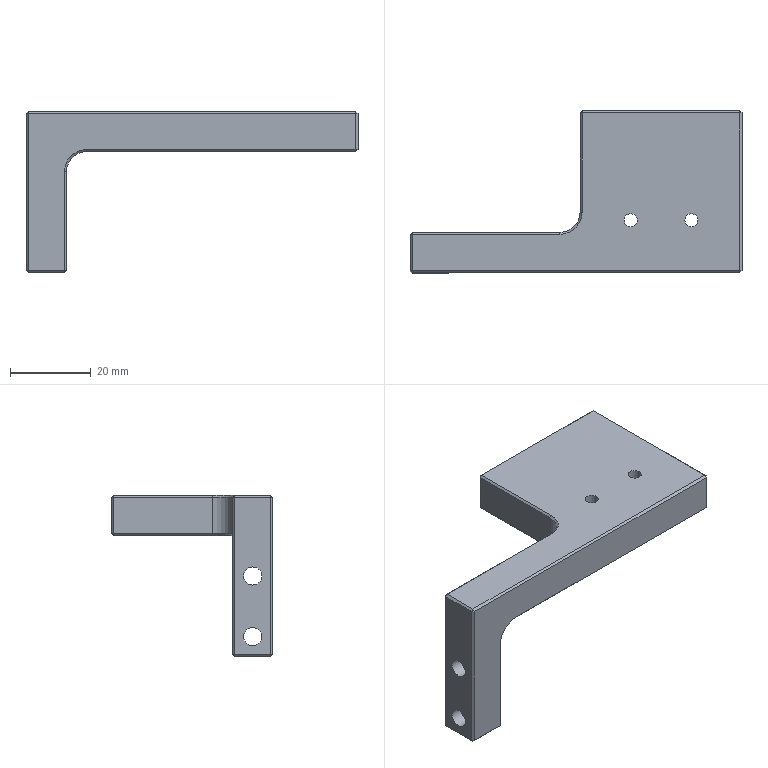Part | 1 solid | 54 faces | box 82 x 40 x 40 mm | volume 22743 mm3 | plane 44 | cylinder 6 | cone 4 | commonest cylinder face diameters 3.242 x2 4.5 x2 10 x2
STEP:
#1=CARTESIAN_POINT('',(11.879,-7.,-10.));
#2=VERTEX_POINT('',#1);
#3=CARTESIAN_POINT('',(13.5,-7.,-10.));
#4=DIRECTION('',(0.,0.,-1.));
#5=DIRECTION('',(-1.,0.,0.));
#6=AXIS2_PLACEMENT_3D('',#3,#4,#5);
#7=CIRCLE('',#6,1.621);
#8=EDGE_CURVE('',#2,#2,#7,.T.);
#9=ORIENTED_EDGE('',*,*,#8,.T.);
#10=EDGE_LOOP('',(#9));
#11=FACE_BOUND('',#10,.T.);
#12=CARTESIAN_POINT('',(15.121,-7.,0.));
#13=VERTEX_POINT('',#12);
#14=CARTESIAN_POINT('',(13.5,-7.,0.));
#15=DIRECTION('',(0.,0.,1.));
#16=DIRECTION('',(1.,0.,0.));
#17=AXIS2_PLACEMENT_3D('',#14,#15,#16);
#18=CIRCLE('',#17,1.621);
#19=EDGE_CURVE('',#13,#13,#18,.T.);
#20=ORIENTED_EDGE('',*,*,#19,.T.);
#21=EDGE_LOOP('',(#20));
#22=FACE_BOUND('',#21,.T.);
#23=CARTESIAN_POINT('',(13.5,-7.,0.));
#24=DIRECTION('',(0.,0.,-1.));
#25=DIRECTION('',(1.,0.,0.));
#26=AXIS2_PLACEMENT_3D('',#23,#24,#25);
#27=CYLINDRICAL_SURFACE('',#26,1.621);
#28=ADVANCED_FACE('',(#11,#22),#27,.F.);
#29=CARTESIAN_POINT('',(1.5,19.5,-10.));
#30=VERTEX_POINT('',#29);
#31=CARTESIAN_POINT('',(1.5,20.,-9.5));
#32=VERTEX_POINT('',#31);
#33=CARTESIAN_POINT('',(1.5,19.75,-9.75));
#34=DIRECTION('',(0.,0.7071,0.7071));
#35=VECTOR('',#34,1000.);
#36=LINE('',#33,#35);
#37=EDGE_CURVE('',#30,#32,#36,.T.);
#38=ORIENTED_EDGE('',*,*,#37,.T.);
#39=CARTESIAN_POINT('',(40.5,20.,-9.5));
#40=VERTEX_POINT('',#39);
#41=CARTESIAN_POINT('',(21.,20.,-9.5));
#42=DIRECTION('',(-1.,0.,0.));
#43=VECTOR('',#42,1000.);
#44=LINE('',#41,#43);
#45=EDGE_CURVE('',#40,#32,#44,.T.);
#46=ORIENTED_EDGE('',*,*,#45,.F.);
#47=CARTESIAN_POINT('',(40.5,19.5,-10.));
#48=VERTEX_POINT('',#47);
#49=CARTESIAN_POINT('',(40.5,19.75,-9.75));
#50=DIRECTION('',(0.,-0.7071,-0.7071));
#51=VECTOR('',#50,1000.);
#52=LINE('',#49,#51);
#53=EDGE_CURVE('',#40,#48,#52,.T.);
#54=ORIENTED_EDGE('',*,*,#53,.T.);
#55=CARTESIAN_POINT('',(21.,19.5,-10.));
#56=DIRECTION('',(-1.,0.,0.));
#57=VECTOR('',#56,1000.);
#58=LINE('',#55,#57);
#59=EDGE_CURVE('',#48,#30,#58,.T.);
#60=ORIENTED_EDGE('',*,*,#59,.T.);
#61=EDGE_LOOP('',(#38,#46,#54,#60));
#62=FACE_BOUND('',#61,.T.);
#63=CARTESIAN_POINT('',(7.25,20.,-9.5));
#64=DIRECTION('',(0.,-0.7071,0.7071));
#65=DIRECTION('',(-1.,0.,0.));
#66=AXIS2_PLACEMENT_3D('',#63,#64,#65);
#67=PLANE('',#66);
#68=ADVANCED_FACE('',(#62),#67,.F.);
#69=CARTESIAN_POINT('',(41.,19.5,-9.5));
#70=VERTEX_POINT('',#69);
#71=CARTESIAN_POINT('',(40.75,19.5,-9.75));
#72=DIRECTION('',(0.7071,0.,0.7071));
#73=VECTOR('',#72,1000.);
#74=LINE('',#71,#73);
#75=EDGE_CURVE('',#48,#70,#74,.T.);
#76=ORIENTED_EDGE('',*,*,#75,.T.);
#77=CARTESIAN_POINT('',(41.,-19.5,-9.5));
#78=VERTEX_POINT('',#77);
#79=CARTESIAN_POINT('',(41.,0.,-9.5));
#80=DIRECTION('',(0.,1.,0.));
#81=VECTOR('',#80,1000.);
#82=LINE('',#79,#81);
#83=EDGE_CURVE('',#78,#70,#82,.T.);
#84=ORIENTED_EDGE('',*,*,#83,.F.);
#85=CARTESIAN_POINT('',(40.5,-19.5,-10.));
#86=VERTEX_POINT('',#85);
#87=CARTESIAN_POINT('',(40.75,-19.5,-9.75));
#88=DIRECTION('',(-0.7071,0.,-0.7071));
#89=VECTOR('',#88,1000.);
#90=LINE('',#87,#89);
#91=EDGE_CURVE('',#78,#86,#90,.T.);
#92=ORIENTED_EDGE('',*,*,#91,.T.);
#93=CARTESIAN_POINT('',(40.5,0.,-10.));
#94=DIRECTION('',(0.,1.,0.));
#95=VECTOR('',#94,1000.);
#96=LINE('',#93,#95);
#97=EDGE_CURVE('',#86,#48,#96,.T.);
#98=ORIENTED_EDGE('',*,*,#97,.T.);
#99=EDGE_LOOP('',(#76,#84,#92,#98));
#100=FACE_BOUND('',#99,.T.);
#101=CARTESIAN_POINT('',(41.,0.25,-9.5));
#102=DIRECTION('',(-0.7071,0.,0.7071));
#103=DIRECTION('',(0.,1.,0.));
#104=AXIS2_PLACEMENT_3D('',#101,#102,#103);
#105=PLANE('',#104);
#106=ADVANCED_FACE('',(#100),#105,.F.);
#107=CARTESIAN_POINT('',(40.5,-20.,-9.5));
#108=VERTEX_POINT('',#107);
#109=CARTESIAN_POINT('',(-26.,-20.,-9.5));
#110=VERTEX_POINT('',#109);
#111=CARTESIAN_POINT('',(7.25,-20.,-9.5));
#112=DIRECTION('',(-1.,0.,0.));
#113=VECTOR('',#112,1000.);
#114=LINE('',#111,#113);
#115=EDGE_CURVE('',#108,#110,#114,.T.);
#116=ORIENTED_EDGE('',*,*,#115,.T.);
#117=CARTESIAN_POINT('',(-26.,-19.5,-10.));
#118=VERTEX_POINT('',#117);
#119=CARTESIAN_POINT('',(-26.,-19.75,-9.75));
#120=DIRECTION('',(0.,-0.7071,0.7071));
#121=VECTOR('',#120,1000.);
#122=LINE('',#119,#121);
#123=EDGE_CURVE('',#118,#110,#122,.T.);
#124=ORIENTED_EDGE('',*,*,#123,.F.);
#125=CARTESIAN_POINT('',(7.25,-19.5,-10.));
#126=DIRECTION('',(-1.,0.,0.));
#127=VECTOR('',#126,1000.);
#128=LINE('',#125,#127);
#129=EDGE_CURVE('',#86,#118,#128,.T.);
#130=ORIENTED_EDGE('',*,*,#129,.F.);
#131=CARTESIAN_POINT('',(40.5,-19.75,-9.75));
#132=DIRECTION('',(0.,-0.7071,0.7071));
#133=VECTOR('',#132,1000.);
#134=LINE('',#131,#133);
#135=EDGE_CURVE('',#86,#108,#134,.T.);
#136=ORIENTED_EDGE('',*,*,#135,.T.);
#137=EDGE_LOOP('',(#116,#124,#130,#136));
#138=FACE_BOUND('',#137,.T.);
#139=CARTESIAN_POINT('',(0.,-20.,-9.5));
#140=DIRECTION('',(0.,-0.7071,-0.7071));
#141=DIRECTION('',(-1.,0.,0.));
#142=AXIS2_PLACEMENT_3D('',#139,#140,#141);
#143=PLANE('',#142);
#144=ADVANCED_FACE('',(#138),#143,.T.);
#145=CARTESIAN_POINT('',(-31.,-10.5,-15.));
#146=VERTEX_POINT('',#145);
#147=CARTESIAN_POINT('',(-26.,-10.5,-10.));
#148=VERTEX_POINT('',#147);
#149=CARTESIAN_POINT('',(-26.,-10.5,-15.));
#150=DIRECTION('',(0.,1.,0.));
#151=DIRECTION('',(1.,0.,0.));
#152=AXIS2_PLACEMENT_3D('',#149,#150,#151);
#153=CIRCLE('',#152,5.);
#154=EDGE_CURVE('',#146,#148,#153,.T.);
#155=ORIENTED_EDGE('',*,*,#154,.T.);
#156=CARTESIAN_POINT('',(-26.,-15.,-10.));
#157=DIRECTION('',(0.,1.,0.));
#158=VECTOR('',#157,1000.);
#159=LINE('',#156,#158);
#160=EDGE_CURVE('',#118,#148,#159,.T.);
#161=ORIENTED_EDGE('',*,*,#160,.F.);
#162=CARTESIAN_POINT('',(-31.,-19.5,-15.));
#163=VERTEX_POINT('',#162);
#164=CARTESIAN_POINT('',(-26.,-19.5,-15.));
#165=DIRECTION('',(0.,1.,0.));
#166=DIRECTION('',(1.,0.,0.));
#167=AXIS2_PLACEMENT_3D('',#164,#165,#166);
#168=CIRCLE('',#167,5.);
#169=EDGE_CURVE('',#163,#118,#168,.T.);
#170=ORIENTED_EDGE('',*,*,#169,.F.);
#171=CARTESIAN_POINT('',(-31.,-15.,-15.));
#172=DIRECTION('',(0.,1.,0.));
#173=VECTOR('',#172,1000.);
#174=LINE('',#171,#173);
#175=EDGE_CURVE('',#163,#146,#174,.T.);
#176=ORIENTED_EDGE('',*,*,#175,.T.);
#177=EDGE_LOOP('',(#155,#161,#170,#176));
#178=FACE_BOUND('',#177,.T.);
#179=CARTESIAN_POINT('',(-26.,0.,-15.));
#180=DIRECTION('',(0.,1.,0.));
#181=DIRECTION('',(-1.,0.,0.));
#182=AXIS2_PLACEMENT_3D('',#179,#180,#181);
#183=CYLINDRICAL_SURFACE('',#182,5.);
#184=ADVANCED_FACE('',(#178),#183,.F.);
#185=CARTESIAN_POINT('',(-4.,-10.,-9.5));
#186=VERTEX_POINT('',#185);
#187=CARTESIAN_POINT('',(-4.,-10.5,-10.));
#188=VERTEX_POINT('',#187);
#189=CARTESIAN_POINT('',(-4.,-10.25,-9.75));
#190=DIRECTION('',(0.,-0.7071,-0.7071));
#191=VECTOR('',#190,1000.);
#192=LINE('',#189,#191);
#193=EDGE_CURVE('',#186,#188,#192,.T.);
#194=ORIENTED_EDGE('',*,*,#193,.T.);
#195=CARTESIAN_POINT('',(-15.,-10.5,-10.));
#196=DIRECTION('',(-1.,0.,0.));
#197=VECTOR('',#196,1000.);
#198=LINE('',#195,#197);
#199=EDGE_CURVE('',#188,#148,#198,.T.);
#200=ORIENTED_EDGE('',*,*,#199,.T.);
#201=CARTESIAN_POINT('',(-26.,-10.,-9.5));
#202=VERTEX_POINT('',#201);
#203=CARTESIAN_POINT('',(-26.,-10.25,-9.75));
#204=DIRECTION('',(0.,0.7071,0.7071));
#205=VECTOR('',#204,1000.);
#206=LINE('',#203,#205);
#207=EDGE_CURVE('',#148,#202,#206,.T.);
#208=ORIENTED_EDGE('',*,*,#207,.T.);
#209=CARTESIAN_POINT('',(-15.,-10.,-9.5));
#210=DIRECTION('',(-1.,0.,0.));
#211=VECTOR('',#210,1000.);
#212=LINE('',#209,#211);
#213=EDGE_CURVE('',#186,#202,#212,.T.);
#214=ORIENTED_EDGE('',*,*,#213,.F.);
#215=EDGE_LOOP('',(#194,#200,#208,#214));
#216=FACE_BOUND('',#215,.T.);
#217=CARTESIAN_POINT('',(2.7,-10.5,-10.));
#218=DIRECTION('',(0.,0.7071,-0.7071));
#219=DIRECTION('',(-1.,0.,0.));
#220=AXIS2_PLACEMENT_3D('',#217,#218,#219);
#221=PLANE('',#220);
#222=ADVANCED_FACE('',(#216),#221,.T.);
#223=CARTESIAN_POINT('',(1.5,-5.,-10.));
#224=VERTEX_POINT('',#223);
#225=CARTESIAN_POINT('',(1.,-5.,-9.5));
#226=VERTEX_POINT('',#225);
#227=CARTESIAN_POINT('',(1.25,-5.,-9.75));
#228=DIRECTION('',(-0.7071,0.,0.7071));
#229=VECTOR('',#228,1000.);
#230=LINE('',#227,#229);
#231=EDGE_CURVE('',#224,#226,#230,.T.);
#232=ORIENTED_EDGE('',*,*,#231,.F.);
#233=CARTESIAN_POINT('',(-4.,-5.,-10.));
#234=DIRECTION('',(0.,0.,-1.));
#235=DIRECTION('',(-1.,0.,0.));
#236=AXIS2_PLACEMENT_3D('',#233,#234,#235);
#237=CIRCLE('',#236,5.5);
#238=EDGE_CURVE('',#224,#188,#237,.T.);
#239=ORIENTED_EDGE('',*,*,#238,.T.);
#240=ORIENTED_EDGE('',*,*,#193,.F.);
#241=CARTESIAN_POINT('',(-4.,-5.,-9.5));
#242=DIRECTION('',(0.,0.,-1.));
#243=DIRECTION('',(-1.,0.,0.));
#244=AXIS2_PLACEMENT_3D('',#241,#242,#243);
#245=CIRCLE('',#244,5.);
#246=EDGE_CURVE('',#226,#186,#245,.T.);
#247=ORIENTED_EDGE('',*,*,#246,.F.);
#248=EDGE_LOOP('',(#232,#239,#240,#247));
#249=FACE_BOUND('',#248,.T.);
#250=CARTESIAN_POINT('',(-4.,-5.,-4.5));
#251=DIRECTION('',(0.,0.,-1.));
#252=DIRECTION('',(0.9659,0.2588,0.));
#253=AXIS2_PLACEMENT_3D('',#250,#251,#252);
#254=CONICAL_SURFACE('',#253,0.,0.7854);
#255=ADVANCED_FACE('',(#249),#254,.F.);
#256=CARTESIAN_POINT('',(1.,19.5,-9.5));
#257=VERTEX_POINT('',#256);
#258=CARTESIAN_POINT('',(1.25,19.5,-9.75));
#259=DIRECTION('',(-0.7071,0.,0.7071));
#260=VECTOR('',#259,1000.);
#261=LINE('',#258,#260);
#262=EDGE_CURVE('',#30,#257,#261,.T.);
#263=ORIENTED_EDGE('',*,*,#262,.F.);
#264=CARTESIAN_POINT('',(1.5,7.25,-10.));
#265=DIRECTION('',(0.,-1.,0.));
#266=VECTOR('',#265,1000.);
#267=LINE('',#264,#266);
#268=EDGE_CURVE('',#30,#224,#267,.T.);
#269=ORIENTED_EDGE('',*,*,#268,.T.);
#270=ORIENTED_EDGE('',*,*,#231,.T.);
#271=CARTESIAN_POINT('',(1.,7.25,-9.5));
#272=DIRECTION('',(0.,-1.,0.));
#273=VECTOR('',#272,1000.);
#274=LINE('',#271,#273);
#275=EDGE_CURVE('',#257,#226,#274,.T.);
#276=ORIENTED_EDGE('',*,*,#275,.F.);
#277=EDGE_LOOP('',(#263,#269,#270,#276));
#278=FACE_BOUND('',#277,.T.);
#279=CARTESIAN_POINT('',(1.5,0.,-10.));
#280=DIRECTION('',(-0.7071,0.,-0.7071));
#281=DIRECTION('',(0.,-1.,0.));
#282=AXIS2_PLACEMENT_3D('',#279,#280,#281);
#283=PLANE('',#282);
#284=ADVANCED_FACE('',(#278),#283,.T.);
#285=CARTESIAN_POINT('',(-40.5,-19.5,0.));
#286=VERTEX_POINT('',#285);
#287=CARTESIAN_POINT('',(-41.,-19.5,-0.5));
#288=VERTEX_POINT('',#287);
#289=CARTESIAN_POINT('',(-40.75,-19.5,-0.25));
#290=DIRECTION('',(-0.7071,0.,-0.7071));
#291=VECTOR('',#290,1000.);
#292=LINE('',#289,#291);
#293=EDGE_CURVE('',#286,#288,#292,.T.);
#294=ORIENTED_EDGE('',*,*,#293,.T.);
#295=CARTESIAN_POINT('',(-40.5,-20.,-0.5));
#296=VERTEX_POINT('',#295);
#297=CARTESIAN_POINT('',(-40.75,-19.75,-0.5));
#298=DIRECTION('',(-0.7071,0.7071,0.));
#299=VECTOR('',#298,1000.);
#300=LINE('',#297,#299);
#301=EDGE_CURVE('',#296,#288,#300,.T.);
#302=ORIENTED_EDGE('',*,*,#301,.F.);
#303=CARTESIAN_POINT('',(-40.5,-19.75,-0.25));
#304=DIRECTION('',(0.,0.7071,0.7071));
#305=VECTOR('',#304,1000.);
#306=LINE('',#303,#305);
#307=EDGE_CURVE('',#296,#286,#306,.T.);
#308=ORIENTED_EDGE('',*,*,#307,.T.);
#309=EDGE_LOOP('',(#294,#302,#308));
#310=FACE_BOUND('',#309,.T.);
#311=CARTESIAN_POINT('',(-40.667,-19.667,-0.3333));
#312=DIRECTION('',(-0.5774,-0.5774,0.5774));
#313=DIRECTION('',(-0.4082,0.8165,0.4082));
#314=AXIS2_PLACEMENT_3D('',#311,#312,#313);
#315=PLANE('',#314);
#316=ADVANCED_FACE('',(#310),#315,.T.);
#317=CARTESIAN_POINT('',(41.,-19.5,-0.5));
#318=VERTEX_POINT('',#317);
#319=CARTESIAN_POINT('',(40.5,-19.5,0.));
#320=VERTEX_POINT('',#319);
#321=CARTESIAN_POINT('',(40.75,-19.5,-0.25));
#322=DIRECTION('',(-0.7071,0.,0.7071));
#323=VECTOR('',#322,1000.);
#324=LINE('',#321,#323);
#325=EDGE_CURVE('',#318,#320,#324,.T.);
#326=ORIENTED_EDGE('',*,*,#325,.T.);
#327=CARTESIAN_POINT('',(40.5,-20.,-0.5));
#328=VERTEX_POINT('',#327);
#329=CARTESIAN_POINT('',(40.5,-19.75,-0.25));
#330=DIRECTION('',(0.,0.7071,0.7071));
#331=VECTOR('',#330,1000.);
#332=LINE('',#329,#331);
#333=EDGE_CURVE('',#328,#320,#332,.T.);
#334=ORIENTED_EDGE('',*,*,#333,.F.);
#335=CARTESIAN_POINT('',(40.75,-19.75,-0.5));
#336=DIRECTION('',(0.7071,0.7071,0.));
#337=VECTOR('',#336,1000.);
#338=LINE('',#335,#337);
#339=EDGE_CURVE('',#328,#318,#338,.T.);
#340=ORIENTED_EDGE('',*,*,#339,.T.);
#341=EDGE_LOOP('',(#326,#334,#340));
#342=FACE_BOUND('',#341,.T.);
#343=CARTESIAN_POINT('',(40.667,-19.667,-0.3333));
#344=DIRECTION('',(-0.5774,0.5774,-0.5774));
#345=DIRECTION('',(0.4082,0.8165,0.4082));
#346=AXIS2_PLACEMENT_3D('',#343,#344,#345);
#347=PLANE('',#346);
#348=ADVANCED_FACE('',(#342),#347,.F.);
#349=CARTESIAN_POINT('',(40.5,20.,-0.5));
#350=VERTEX_POINT('',#349);
#351=CARTESIAN_POINT('',(40.5,19.5,0.));
#352=VERTEX_POINT('',#351);
#353=CARTESIAN_POINT('',(40.5,19.75,-0.25));
#354=DIRECTION('',(0.,-0.7071,0.7071));
#355=VECTOR('',#354,1000.);
#356=LINE('',#353,#355);
#357=EDGE_CURVE('',#350,#352,#356,.T.);
#358=ORIENTED_EDGE('',*,*,#357,.T.);
#359=CARTESIAN_POINT('',(41.,19.5,-0.5));
#360=VERTEX_POINT('',#359);
#361=CARTESIAN_POINT('',(40.75,19.5,-0.25));
#362=DIRECTION('',(-0.7071,0.,0.7071));
#363=VECTOR('',#362,1000.);
#364=LINE('',#361,#363);
#365=EDGE_CURVE('',#360,#352,#364,.T.);
#366=ORIENTED_EDGE('',*,*,#365,.F.);
#367=CARTESIAN_POINT('',(40.75,19.75,-0.5));
#368=DIRECTION('',(-0.7071,0.7071,0.));
#369=VECTOR('',#368,1000.);
#370=LINE('',#367,#369);
#371=EDGE_CURVE('',#360,#350,#370,.T.);
#372=ORIENTED_EDGE('',*,*,#371,.T.);
#373=EDGE_LOOP('',(#358,#366,#372));
#374=FACE_BOUND('',#373,.T.);
#375=CARTESIAN_POINT('',(40.667,19.667,-0.3333));
#376=DIRECTION('',(-0.5774,-0.5774,-0.5774));
#377=DIRECTION('',(-0.4082,0.8165,-0.4082));
#378=AXIS2_PLACEMENT_3D('',#375,#376,#377);
#379=PLANE('',#378);
#380=ADVANCED_FACE('',(#374),#379,.F.);
#381=CARTESIAN_POINT('',(1.5,19.5,0.));
#382=VERTEX_POINT('',#381);
#383=CARTESIAN_POINT('',(1.,19.5,-0.5));
#384=VERTEX_POINT('',#383);
#385=CARTESIAN_POINT('',(1.25,19.5,-0.25));
#386=DIRECTION('',(-0.7071,0.,-0.7071));
#387=VECTOR('',#386,1000.);
#388=LINE('',#385,#387);
#389=EDGE_CURVE('',#382,#384,#388,.T.);
#390=ORIENTED_EDGE('',*,*,#389,.F.);
#391=CARTESIAN_POINT('',(1.5,20.,-0.5));
#392=VERTEX_POINT('',#391);
#393=CARTESIAN_POINT('',(1.5,19.75,-0.25));
#394=DIRECTION('',(0.,-0.7071,0.7071));
#395=VECTOR('',#394,1000.);
#396=LINE('',#393,#395);
#397=EDGE_CURVE('',#392,#382,#396,.T.);
#398=ORIENTED_EDGE('',*,*,#397,.F.);
#399=CARTESIAN_POINT('',(1.25,19.75,-0.5));
#400=DIRECTION('',(-0.7071,-0.7071,0.));
#401=VECTOR('',#400,1000.);
#402=LINE('',#399,#401);
#403=EDGE_CURVE('',#392,#384,#402,.T.);
#404=ORIENTED_EDGE('',*,*,#403,.T.);
#405=EDGE_LOOP('',(#390,#398,#404));
#406=FACE_BOUND('',#405,.T.);
#407=CARTESIAN_POINT('',(1.333,19.667,-0.3333));
#408=DIRECTION('',(0.5774,-0.5774,-0.5774));
#409=DIRECTION('',(0.4082,0.8165,-0.4082));
#410=AXIS2_PLACEMENT_3D('',#407,#408,#409);
#411=PLANE('',#410);
#412=ADVANCED_FACE('',(#406),#411,.F.);
#413=CARTESIAN_POINT('',(-41.,-15.,-22.25));
#414=VERTEX_POINT('',#413);
#415=CARTESIAN_POINT('',(-41.,-15.,-20.));
#416=DIRECTION('',(1.,0.,0.));
#417=DIRECTION('',(0.,0.,-1.));
#418=AXIS2_PLACEMENT_3D('',#415,#416,#417);
#419=CIRCLE('',#418,2.25);
#420=EDGE_CURVE('',#414,#414,#419,.T.);
#421=ORIENTED_EDGE('',*,*,#420,.F.);
#422=EDGE_LOOP('',(#421));
#423=FACE_BOUND('',#422,.T.);
#424=CARTESIAN_POINT('',(-31.,-15.,-22.25));
#425=VERTEX_POINT('',#424);
#426=CARTESIAN_POINT('',(-31.,-15.,-20.));
#427=DIRECTION('',(1.,0.,0.));
#428=DIRECTION('',(0.,0.,-1.));
#429=AXIS2_PLACEMENT_3D('',#426,#427,#428);
#430=CIRCLE('',#429,2.25);
#431=EDGE_CURVE('',#425,#425,#430,.T.);
#432=ORIENTED_EDGE('',*,*,#431,.T.);
#433=EDGE_LOOP('',(#432));
#434=FACE_BOUND('',#433,.T.);
#435=CARTESIAN_POINT('',(0.66,-15.,-20.));
#436=DIRECTION('',(-1.,0.,0.));
#437=DIRECTION('',(0.,-1.,0.));
#438=AXIS2_PLACEMENT_3D('',#435,#436,#437);
#439=CYLINDRICAL_SURFACE('',#438,2.25);
#440=ADVANCED_FACE('',(#423,#434),#439,.F.);
#441=CARTESIAN_POINT('',(-41.,-15.,-37.25));
#442=VERTEX_POINT('',#441);
#443=CARTESIAN_POINT('',(-41.,-15.,-35.));
#444=DIRECTION('',(1.,0.,0.));
#445=DIRECTION('',(0.,0.,-1.));
#446=AXIS2_PLACEMENT_3D('',#443,#444,#445);
#447=CIRCLE('',#446,2.25);
#448=EDGE_CURVE('',#442,#442,#447,.T.);
#449=ORIENTED_EDGE('',*,*,#448,.F.);
#450=EDGE_LOOP('',(#449));
#451=FACE_BOUND('',#450,.T.);
#452=CARTESIAN_POINT('',(-31.,-15.,-37.25));
#453=VERTEX_POINT('',#452);
#454=CARTESIAN_POINT('',(-31.,-15.,-35.));
#455=DIRECTION('',(1.,0.,0.));
#456=DIRECTION('',(0.,0.,-1.));
#457=AXIS2_PLACEMENT_3D('',#454,#455,#456);
#458=CIRCLE('',#457,2.25);
#459=EDGE_CURVE('',#453,#453,#458,.T.);
#460=ORIENTED_EDGE('',*,*,#459,.T.);
#461=EDGE_LOOP('',(#460));
#462=FACE_BOUND('',#461,.T.);
#463=CARTESIAN_POINT('',(0.66,-15.,-35.));
#464=DIRECTION('',(-1.,0.,0.));
#465=DIRECTION('',(0.,-1.,0.));
#466=AXIS2_PLACEMENT_3D('',#463,#464,#465);
#467=CYLINDRICAL_SURFACE('',#466,2.25);
#468=ADVANCED_FACE('',(#451,#462),#467,.F.);
#469=CARTESIAN_POINT('',(1.5,20.,-5.));
#470=DIRECTION('',(0.,0.,-1.));
#471=VECTOR('',#470,1000.);
#472=LINE('',#469,#471);
#473=EDGE_CURVE('',#392,#32,#472,.T.);
#474=ORIENTED_EDGE('',*,*,#473,.T.);
#475=CARTESIAN_POINT('',(1.25,19.75,-9.5));
#476=DIRECTION('',(0.7071,0.7071,0.));
#477=VECTOR('',#476,1000.);
#478=LINE('',#475,#477);
#479=EDGE_CURVE('',#257,#32,#478,.T.);
#480=ORIENTED_EDGE('',*,*,#479,.F.);
#481=CARTESIAN_POINT('',(1.,19.5,-5.));
#482=DIRECTION('',(0.,0.,-1.));
#483=VECTOR('',#482,1000.);
#484=LINE('',#481,#483);
#485=EDGE_CURVE('',#384,#257,#484,.T.);
#486=ORIENTED_EDGE('',*,*,#485,.F.);
#487=ORIENTED_EDGE('',*,*,#403,.F.);
#488=EDGE_LOOP('',(#474,#480,#486,#487));
#489=FACE_BOUND('',#488,.T.);
#490=CARTESIAN_POINT('',(1.5,20.,-5.));
#491=DIRECTION('',(-0.7071,0.7071,0.));
#492=DIRECTION('',(0.,0.,-1.));
#493=AXIS2_PLACEMENT_3D('',#490,#491,#492);
#494=PLANE('',#493);
#495=ADVANCED_FACE('',(#489),#494,.T.);
#496=CARTESIAN_POINT('',(-40.5,-10.5,-40.));
#497=VERTEX_POINT('',#496);
#498=CARTESIAN_POINT('',(-31.5,-10.5,-40.));
#499=VERTEX_POINT('',#498);
#500=CARTESIAN_POINT('',(-36.,-10.5,-40.));
#501=DIRECTION('',(1.,0.,0.));
#502=VECTOR('',#501,1000.);
#503=LINE('',#500,#502);
#504=EDGE_CURVE('',#497,#499,#503,.T.);
#505=ORIENTED_EDGE('',*,*,#504,.F.);
#506=CARTESIAN_POINT('',(-40.5,-10.,-39.5));
#507=VERTEX_POINT('',#506);
#508=CARTESIAN_POINT('',(-40.5,-10.25,-39.75));
#509=DIRECTION('',(0.,-0.7071,-0.7071));
#510=VECTOR('',#509,1000.);
#511=LINE('',#508,#510);
#512=EDGE_CURVE('',#507,#497,#511,.T.);
#513=ORIENTED_EDGE('',*,*,#512,.F.);
#514=CARTESIAN_POINT('',(-31.5,-10.,-39.5));
#515=VERTEX_POINT('',#514);
#516=CARTESIAN_POINT('',(-36.,-10.,-39.5));
#517=DIRECTION('',(1.,0.,0.));
#518=VECTOR('',#517,1000.);
#519=LINE('',#516,#518);
#520=EDGE_CURVE('',#507,#515,#519,.T.);
#521=ORIENTED_EDGE('',*,*,#520,.T.);
#522=CARTESIAN_POINT('',(-31.5,-10.25,-39.75));
#523=DIRECTION('',(0.,0.7071,0.7071));
#524=VECTOR('',#523,1000.);
#525=LINE('',#522,#524);
#526=EDGE_CURVE('',#499,#515,#525,.T.);
#527=ORIENTED_EDGE('',*,*,#526,.F.);
#528=EDGE_LOOP('',(#505,#513,#521,#527));
#529=FACE_BOUND('',#528,.T.);
#530=CARTESIAN_POINT('',(-22.25,-10.,-39.5));
#531=DIRECTION('',(0.,0.7071,-0.7071));
#532=DIRECTION('',(1.,0.,0.));
#533=AXIS2_PLACEMENT_3D('',#530,#531,#532);
#534=PLANE('',#533);
#535=ADVANCED_FACE('',(#529),#534,.T.);
#536=ORIENTED_EDGE('',*,*,#512,.T.);
#537=CARTESIAN_POINT('',(-41.,-10.5,-39.5));
#538=VERTEX_POINT('',#537);
#539=CARTESIAN_POINT('',(-40.75,-10.5,-39.75));
#540=DIRECTION('',(-0.7071,0.,0.7071));
#541=VECTOR('',#540,1000.);
#542=LINE('',#539,#541);
#543=EDGE_CURVE('',#497,#538,#542,.T.);
#544=ORIENTED_EDGE('',*,*,#543,.T.);
#545=CARTESIAN_POINT('',(-40.75,-10.25,-39.5));
#546=DIRECTION('',(-0.7071,-0.7071,0.));
#547=VECTOR('',#546,1000.);
#548=LINE('',#545,#547);
#549=EDGE_CURVE('',#507,#538,#548,.T.);
#550=ORIENTED_EDGE('',*,*,#549,.F.);
#551=EDGE_LOOP('',(#536,#544,#550));
#552=FACE_BOUND('',#551,.T.);
#553=CARTESIAN_POINT('',(-40.667,-10.333,-39.667));
#554=DIRECTION('',(0.5774,-0.5774,0.5774));
#555=DIRECTION('',(0.4082,0.8165,0.4082));
#556=AXIS2_PLACEMENT_3D('',#553,#554,#555);
#557=PLANE('',#556);
#558=ADVANCED_FACE('',(#552),#557,.F.);
#559=CARTESIAN_POINT('',(-31.5,-19.5,-40.));
#560=VERTEX_POINT('',#559);
#561=CARTESIAN_POINT('',(-31.,-19.5,-39.5));
#562=VERTEX_POINT('',#561);
#563=CARTESIAN_POINT('',(-31.25,-19.5,-39.75));
#564=DIRECTION('',(0.7071,0.,0.7071));
#565=VECTOR('',#564,1000.);
#566=LINE('',#563,#565);
#567=EDGE_CURVE('',#560,#562,#566,.T.);
#568=ORIENTED_EDGE('',*,*,#567,.T.);
#569=CARTESIAN_POINT('',(-31.5,-20.,-39.5));
#570=VERTEX_POINT('',#569);
#571=CARTESIAN_POINT('',(-31.25,-19.75,-39.5));
#572=DIRECTION('',(0.7071,0.7071,0.));
#573=VECTOR('',#572,1000.);
#574=LINE('',#571,#573);
#575=EDGE_CURVE('',#570,#562,#574,.T.);
#576=ORIENTED_EDGE('',*,*,#575,.F.);
#577=CARTESIAN_POINT('',(-31.5,-19.75,-39.75));
#578=DIRECTION('',(0.,0.7071,-0.7071));
#579=VECTOR('',#578,1000.);
#580=LINE('',#577,#579);
#581=EDGE_CURVE('',#570,#560,#580,.T.);
#582=ORIENTED_EDGE('',*,*,#581,.T.);
#583=EDGE_LOOP('',(#568,#576,#582));
#584=FACE_BOUND('',#583,.T.);
#585=CARTESIAN_POINT('',(-31.333,-19.667,-39.667));
#586=DIRECTION('',(-0.5774,0.5774,0.5774));
#587=DIRECTION('',(0.4082,0.8165,-0.4082));
#588=AXIS2_PLACEMENT_3D('',#585,#586,#587);
#589=PLANE('',#588);
#590=ADVANCED_FACE('',(#584),#589,.F.);
#591=ORIENTED_EDGE('',*,*,#91,.F.);
#592=CARTESIAN_POINT('',(40.75,-19.75,-9.5));
#593=DIRECTION('',(0.7071,0.7071,0.));
#594=VECTOR('',#593,1000.);
#595=LINE('',#592,#594);
#596=EDGE_CURVE('',#108,#78,#595,.T.);
#597=ORIENTED_EDGE('',*,*,#596,.F.);
#598=ORIENTED_EDGE('',*,*,#135,.F.);
#599=EDGE_LOOP('',(#591,#597,#598));
#600=FACE_BOUND('',#599,.T.);
#601=CARTESIAN_POINT('',(40.667,-19.667,-9.667));
#602=DIRECTION('',(-0.5774,0.5774,0.5774));
#603=DIRECTION('',(0.4082,0.8165,-0.4082));
#604=AXIS2_PLACEMENT_3D('',#601,#602,#603);
#605=PLANE('',#604);
#606=ADVANCED_FACE('',(#600),#605,.F.);
#607=ORIENTED_EDGE('',*,*,#53,.F.);
#608=CARTESIAN_POINT('',(40.75,19.75,-9.5));
#609=DIRECTION('',(-0.7071,0.7071,0.));
#610=VECTOR('',#609,1000.);
#611=LINE('',#608,#610);
#612=EDGE_CURVE('',#70,#40,#611,.T.);
#613=ORIENTED_EDGE('',*,*,#612,.F.);
#614=ORIENTED_EDGE('',*,*,#75,.F.);
#615=EDGE_LOOP('',(#607,#613,#614));
#616=FACE_BOUND('',#615,.T.);
#617=CARTESIAN_POINT('',(40.667,19.667,-9.667));
#618=DIRECTION('',(-0.5774,-0.5774,0.5774));
#619=DIRECTION('',(-0.4082,0.8165,0.4082));
#620=AXIS2_PLACEMENT_3D('',#617,#618,#619);
#621=PLANE('',#620);
#622=ADVANCED_FACE('',(#616),#621,.F.);
#623=ORIENTED_EDGE('',*,*,#567,.F.);
#624=CARTESIAN_POINT('',(-31.5,-15.,-40.));
#625=DIRECTION('',(0.,1.,0.));
#626=VECTOR('',#625,1000.);
#627=LINE('',#624,#626);
#628=EDGE_CURVE('',#560,#499,#627,.T.);
#629=ORIENTED_EDGE('',*,*,#628,.T.);
#630=CARTESIAN_POINT('',(-31.,-10.5,-39.5));
#631=VERTEX_POINT('',#630);
#632=CARTESIAN_POINT('',(-31.25,-10.5,-39.75));
#633=DIRECTION('',(0.7071,0.,0.7071));
#634=VECTOR('',#633,1000.);
#635=LINE('',#632,#634);
#636=EDGE_CURVE('',#499,#631,#635,.T.);
#637=ORIENTED_EDGE('',*,*,#636,.T.);
#638=CARTESIAN_POINT('',(-31.,-15.,-39.5));
#639=DIRECTION('',(0.,1.,0.));
#640=VECTOR('',#639,1000.);
#641=LINE('',#638,#640);
#642=EDGE_CURVE('',#562,#631,#641,.T.);
#643=ORIENTED_EDGE('',*,*,#642,.F.);
#644=EDGE_LOOP('',(#623,#629,#637,#643));
#645=FACE_BOUND('',#644,.T.);
#646=CARTESIAN_POINT('',(-31.5,-15.,-40.));
#647=DIRECTION('',(0.7071,0.,-0.7071));
#648=DIRECTION('',(0.,1.,0.));
#649=AXIS2_PLACEMENT_3D('',#646,#647,#648);
#650=PLANE('',#649);
#651=ADVANCED_FACE('',(#645),#650,.T.);
#652=ORIENTED_EDGE('',*,*,#262,.T.);
#653=ORIENTED_EDGE('',*,*,#479,.T.);
#654=ORIENTED_EDGE('',*,*,#37,.F.);
#655=EDGE_LOOP('',(#652,#653,#654));
#656=FACE_BOUND('',#655,.T.);
#657=CARTESIAN_POINT('',(1.333,19.667,-9.667));
#658=DIRECTION('',(0.5774,-0.5774,0.5774));
#659=DIRECTION('',(0.4082,0.8165,0.4082));
#660=AXIS2_PLACEMENT_3D('',#657,#658,#659);
#661=PLANE('',#660);
#662=ADVANCED_FACE('',(#656),#661,.F.);
#663=ORIENTED_EDGE('',*,*,#636,.F.);
#664=ORIENTED_EDGE('',*,*,#526,.T.);
#665=CARTESIAN_POINT('',(-31.25,-10.25,-39.5));
#666=DIRECTION('',(-0.7071,0.7071,0.));
#667=VECTOR('',#666,1000.);
#668=LINE('',#665,#667);
#669=EDGE_CURVE('',#631,#515,#668,.T.);
#670=ORIENTED_EDGE('',*,*,#669,.F.);
#671=EDGE_LOOP('',(#663,#664,#670));
#672=FACE_BOUND('',#671,.T.);
#673=CARTESIAN_POINT('',(-31.333,-10.333,-39.667));
#674=DIRECTION('',(-0.5774,-0.5774,0.5774));
#675=DIRECTION('',(-0.4082,0.8165,0.4082));
#676=AXIS2_PLACEMENT_3D('',#673,#674,#675);
#677=PLANE('',#676);
#678=ADVANCED_FACE('',(#672),#677,.F.);
#679=ORIENTED_EDGE('',*,*,#459,.F.);
#680=EDGE_LOOP('',(#679));
#681=FACE_BOUND('',#680,.T.);
#682=ORIENTED_EDGE('',*,*,#431,.F.);
#683=EDGE_LOOP('',(#682));
#684=FACE_BOUND('',#683,.T.);
#685=CARTESIAN_POINT('',(-31.,-10.5,-20.));
#686=DIRECTION('',(0.,0.,-1.));
#687=VECTOR('',#686,1000.);
#688=LINE('',#685,#687);
#689=EDGE_CURVE('',#146,#631,#688,.T.);
#690=ORIENTED_EDGE('',*,*,#689,.F.);
#691=ORIENTED_EDGE('',*,*,#175,.F.);
#692=CARTESIAN_POINT('',(-31.,-19.5,-20.));
#693=DIRECTION('',(0.,0.,-1.));
#694=VECTOR('',#693,1000.);
#695=LINE('',#692,#694);
#696=EDGE_CURVE('',#163,#562,#695,.T.);
#697=ORIENTED_EDGE('',*,*,#696,.T.);
#698=ORIENTED_EDGE('',*,*,#642,.T.);
#699=EDGE_LOOP('',(#690,#691,#697,#698));
#700=FACE_BOUND('',#699,.T.);
#701=CARTESIAN_POINT('',(-31.,-20.,-10.));
#702=DIRECTION('',(1.,0.,0.));
#703=DIRECTION('',(0.,0.,-1.));
#704=AXIS2_PLACEMENT_3D('',#701,#702,#703);
#705=PLANE('',#704);
#706=ADVANCED_FACE('',(#681,#684,#700),#705,.T.);
#707=ORIENTED_EDGE('',*,*,#628,.F.);
#708=CARTESIAN_POINT('',(-40.5,-19.5,-40.));
#709=VERTEX_POINT('',#708);
#710=CARTESIAN_POINT('',(0.,-19.5,-40.));
#711=DIRECTION('',(-1.,0.,0.));
#712=VECTOR('',#711,1000.);
#713=LINE('',#710,#712);
#714=EDGE_CURVE('',#560,#709,#713,.T.);
#715=ORIENTED_EDGE('',*,*,#714,.T.);
#716=CARTESIAN_POINT('',(-40.5,-14.75,-40.));
#717=DIRECTION('',(0.,1.,0.));
#718=VECTOR('',#717,1000.);
#719=LINE('',#716,#718);
#720=EDGE_CURVE('',#709,#497,#719,.T.);
#721=ORIENTED_EDGE('',*,*,#720,.T.);
#722=ORIENTED_EDGE('',*,*,#504,.T.);
#723=EDGE_LOOP('',(#707,#715,#721,#722));
#724=FACE_BOUND('',#723,.T.);
#725=CARTESIAN_POINT('',(0.,0.,-40.));
#726=DIRECTION('',(0.,0.,1.));
#727=DIRECTION('',(1.,0.,0.));
#728=AXIS2_PLACEMENT_3D('',#725,#726,#727);
#729=PLANE('',#728);
#730=ADVANCED_FACE('',(#724),#729,.F.);
#731=CARTESIAN_POINT('',(-41.,-19.5,-39.5));
#732=VERTEX_POINT('',#731);
#733=CARTESIAN_POINT('',(-40.75,-19.5,-39.75));
#734=DIRECTION('',(-0.7071,0.,0.7071));
#735=VECTOR('',#734,1000.);
#736=LINE('',#733,#735);
#737=EDGE_CURVE('',#709,#732,#736,.T.);
#738=ORIENTED_EDGE('',*,*,#737,.F.);
#739=CARTESIAN_POINT('',(-40.5,-20.,-39.5));
#740=VERTEX_POINT('',#739);
#741=CARTESIAN_POINT('',(-40.5,-19.75,-39.75));
#742=DIRECTION('',(0.,0.7071,-0.7071));
#743=VECTOR('',#742,1000.);
#744=LINE('',#741,#743);
#745=EDGE_CURVE('',#740,#709,#744,.T.);
#746=ORIENTED_EDGE('',*,*,#745,.F.);
#747=CARTESIAN_POINT('',(-40.75,-19.75,-39.5));
#748=DIRECTION('',(-0.7071,0.7071,0.));
#749=VECTOR('',#748,1000.);
#750=LINE('',#747,#749);
#751=EDGE_CURVE('',#740,#732,#750,.T.);
#752=ORIENTED_EDGE('',*,*,#751,.T.);
#753=EDGE_LOOP('',(#738,#746,#752));
#754=FACE_BOUND('',#753,.T.);
#755=CARTESIAN_POINT('',(-40.667,-19.667,-39.667));
#756=DIRECTION('',(0.5774,0.5774,0.5774));
#757=DIRECTION('',(-0.4082,0.8165,-0.4082));
#758=AXIS2_PLACEMENT_3D('',#755,#756,#757);
#759=PLANE('',#758);
#760=ADVANCED_FACE('',(#754),#759,.F.);
#761=CARTESIAN_POINT('',(-31.5,-10.,-15.));
#762=VERTEX_POINT('',#761);
#763=CARTESIAN_POINT('',(-31.5,-10.,-27.25));
#764=DIRECTION('',(0.,0.,-1.));
#765=VECTOR('',#764,1000.);
#766=LINE('',#763,#765);
#767=EDGE_CURVE('',#762,#515,#766,.T.);
#768=ORIENTED_EDGE('',*,*,#767,.F.);
#769=CARTESIAN_POINT('',(-31.25,-10.25,-15.));
#770=DIRECTION('',(-0.7071,0.7071,0.));
#771=VECTOR('',#770,1000.);
#772=LINE('',#769,#771);
#773=EDGE_CURVE('',#146,#762,#772,.T.);
#774=ORIENTED_EDGE('',*,*,#773,.F.);
#775=ORIENTED_EDGE('',*,*,#689,.T.);
#776=ORIENTED_EDGE('',*,*,#669,.T.);
#777=EDGE_LOOP('',(#768,#774,#775,#776));
#778=FACE_BOUND('',#777,.T.);
#779=CARTESIAN_POINT('',(-31.,-10.5,-20.));
#780=DIRECTION('',(0.7071,0.7071,0.));
#781=DIRECTION('',(0.,0.,-1.));
#782=AXIS2_PLACEMENT_3D('',#779,#780,#781);
#783=PLANE('',#782);
#784=ADVANCED_FACE('',(#778),#783,.T.);
#785=ORIENTED_EDGE('',*,*,#207,.F.);
#786=ORIENTED_EDGE('',*,*,#154,.F.);
#787=ORIENTED_EDGE('',*,*,#773,.T.);
#788=CARTESIAN_POINT('',(-26.,-10.,-15.));
#789=DIRECTION('',(0.,1.,0.));
#790=DIRECTION('',(1.,0.,0.));
#791=AXIS2_PLACEMENT_3D('',#788,#789,#790);
#792=CIRCLE('',#791,5.5);
#793=EDGE_CURVE('',#762,#202,#792,.T.);
#794=ORIENTED_EDGE('',*,*,#793,.T.);
#795=EDGE_LOOP('',(#785,#786,#787,#794));
#796=FACE_BOUND('',#795,.T.);
#797=CARTESIAN_POINT('',(-26.,-15.5,-15.));
#798=DIRECTION('',(0.,1.,0.));
#799=DIRECTION('',(-0.9659,0.,-0.2588));
#800=AXIS2_PLACEMENT_3D('',#797,#798,#799);
#801=CONICAL_SURFACE('',#800,0.,0.7854);
#802=ADVANCED_FACE('',(#796),#801,.F.);
#803=ORIENTED_EDGE('',*,*,#371,.F.);
#804=CARTESIAN_POINT('',(41.,19.5,-5.));
#805=DIRECTION('',(0.,0.,1.));
#806=VECTOR('',#805,1000.);
#807=LINE('',#804,#806);
#808=EDGE_CURVE('',#70,#360,#807,.T.);
#809=ORIENTED_EDGE('',*,*,#808,.F.);
#810=ORIENTED_EDGE('',*,*,#612,.T.);
#811=CARTESIAN_POINT('',(40.5,20.,-5.));
#812=DIRECTION('',(0.,0.,1.));
#813=VECTOR('',#812,1000.);
#814=LINE('',#811,#813);
#815=EDGE_CURVE('',#40,#350,#814,.T.);
#816=ORIENTED_EDGE('',*,*,#815,.T.);
#817=EDGE_LOOP('',(#803,#809,#810,#816));
#818=FACE_BOUND('',#817,.T.);
#819=CARTESIAN_POINT('',(41.,19.5,-5.));
#820=DIRECTION('',(-0.7071,-0.7071,0.));
#821=DIRECTION('',(0.,0.,1.));
#822=AXIS2_PLACEMENT_3D('',#819,#820,#821);
#823=PLANE('',#822);
#824=ADVANCED_FACE('',(#818),#823,.F.);
#825=ORIENTED_EDGE('',*,*,#596,.T.);
#826=CARTESIAN_POINT('',(41.,-19.5,-5.));
#827=DIRECTION('',(0.,0.,1.));
#828=VECTOR('',#827,1000.);
#829=LINE('',#826,#828);
#830=EDGE_CURVE('',#78,#318,#829,.T.);
#831=ORIENTED_EDGE('',*,*,#830,.T.);
#832=ORIENTED_EDGE('',*,*,#339,.F.);
#833=CARTESIAN_POINT('',(40.5,-20.,-5.));
#834=DIRECTION('',(0.,0.,1.));
#835=VECTOR('',#834,1000.);
#836=LINE('',#833,#835);
#837=EDGE_CURVE('',#108,#328,#836,.T.);
#838=ORIENTED_EDGE('',*,*,#837,.F.);
#839=EDGE_LOOP('',(#825,#831,#832,#838));
#840=FACE_BOUND('',#839,.T.);
#841=CARTESIAN_POINT('',(40.5,-20.,-20.));
#842=DIRECTION('',(-0.7071,0.7071,0.));
#843=DIRECTION('',(0.,0.,1.));
#844=AXIS2_PLACEMENT_3D('',#841,#842,#843);
#845=PLANE('',#844);
#846=ADVANCED_FACE('',(#840),#845,.F.);
#847=CARTESIAN_POINT('',(-36.,-20.,-39.5));
#848=DIRECTION('',(-1.,0.,0.));
#849=VECTOR('',#848,1000.);
#850=LINE('',#847,#849);
#851=EDGE_CURVE('',#570,#740,#850,.T.);
#852=ORIENTED_EDGE('',*,*,#851,.T.);
#853=ORIENTED_EDGE('',*,*,#745,.T.);
#854=ORIENTED_EDGE('',*,*,#714,.F.);
#855=ORIENTED_EDGE('',*,*,#581,.F.);
#856=EDGE_LOOP('',(#852,#853,#854,#855));
#857=FACE_BOUND('',#856,.T.);
#858=CARTESIAN_POINT('',(0.,-20.,-39.5));
#859=DIRECTION('',(0.,-0.7071,-0.7071));
#860=DIRECTION('',(-1.,0.,0.));
#861=AXIS2_PLACEMENT_3D('',#858,#859,#860);
#862=PLANE('',#861);
#863=ADVANCED_FACE('',(#857),#862,.T.);
#864=ORIENTED_EDGE('',*,*,#696,.F.);
#865=CARTESIAN_POINT('',(-31.5,-20.,-15.));
#866=VERTEX_POINT('',#865);
#867=CARTESIAN_POINT('',(-31.25,-19.75,-15.));
#868=DIRECTION('',(-0.7071,-0.7071,0.));
#869=VECTOR('',#868,1000.);
#870=LINE('',#867,#869);
#871=EDGE_CURVE('',#163,#866,#870,.T.);
#872=ORIENTED_EDGE('',*,*,#871,.T.);
#873=CARTESIAN_POINT('',(-31.5,-20.,-27.25));
#874=DIRECTION('',(0.,0.,-1.));
#875=VECTOR('',#874,1000.);
#876=LINE('',#873,#875);
#877=EDGE_CURVE('',#866,#570,#876,.T.);
#878=ORIENTED_EDGE('',*,*,#877,.T.);
#879=ORIENTED_EDGE('',*,*,#575,.T.);
#880=EDGE_LOOP('',(#864,#872,#878,#879));
#881=FACE_BOUND('',#880,.T.);
#882=CARTESIAN_POINT('',(-31.5,-20.,-20.));
#883=DIRECTION('',(0.7071,-0.7071,0.));
#884=DIRECTION('',(0.,0.,-1.));
#885=AXIS2_PLACEMENT_3D('',#882,#883,#884);
#886=PLANE('',#885);
#887=ADVANCED_FACE('',(#881),#886,.T.);
#888=ORIENTED_EDGE('',*,*,#871,.F.);
#889=ORIENTED_EDGE('',*,*,#169,.T.);
#890=ORIENTED_EDGE('',*,*,#123,.T.);
#891=CARTESIAN_POINT('',(-26.,-20.,-15.));
#892=DIRECTION('',(0.,1.,0.));
#893=DIRECTION('',(1.,0.,0.));
#894=AXIS2_PLACEMENT_3D('',#891,#892,#893);
#895=CIRCLE('',#894,5.5);
#896=EDGE_CURVE('',#866,#110,#895,.T.);
#897=ORIENTED_EDGE('',*,*,#896,.F.);
#898=EDGE_LOOP('',(#888,#889,#890,#897));
#899=FACE_BOUND('',#898,.T.);
#900=CARTESIAN_POINT('',(-26.,-14.5,-15.));
#901=DIRECTION('',(0.,-1.,0.));
#902=DIRECTION('',(-0.9659,0.,-0.2588));
#903=AXIS2_PLACEMENT_3D('',#900,#901,#902);
#904=CONICAL_SURFACE('',#903,0.,0.7854);
#905=ADVANCED_FACE('',(#899),#904,.F.);
#906=CARTESIAN_POINT('',(-41.,-10.5,-0.5));
#907=VERTEX_POINT('',#906);
#908=CARTESIAN_POINT('',(-41.,-10.5,-20.));
#909=DIRECTION('',(0.,0.,-1.));
#910=VECTOR('',#909,1000.);
#911=LINE('',#908,#910);
#912=EDGE_CURVE('',#907,#538,#911,.T.);
#913=ORIENTED_EDGE('',*,*,#912,.F.);
#914=CARTESIAN_POINT('',(-40.5,-10.,-0.5));
#915=VERTEX_POINT('',#914);
#916=CARTESIAN_POINT('',(-40.75,-10.25,-0.5));
#917=DIRECTION('',(-0.7071,-0.7071,0.));
#918=VECTOR('',#917,1000.);
#919=LINE('',#916,#918);
#920=EDGE_CURVE('',#915,#907,#919,.T.);
#921=ORIENTED_EDGE('',*,*,#920,.F.);
#922=CARTESIAN_POINT('',(-40.5,-10.,-20.));
#923=DIRECTION('',(0.,0.,-1.));
#924=VECTOR('',#923,1000.);
#925=LINE('',#922,#924);
#926=EDGE_CURVE('',#915,#507,#925,.T.);
#927=ORIENTED_EDGE('',*,*,#926,.T.);
#928=ORIENTED_EDGE('',*,*,#549,.T.);
#929=EDGE_LOOP('',(#913,#921,#927,#928));
#930=FACE_BOUND('',#929,.T.);
#931=CARTESIAN_POINT('',(-40.5,-10.,-20.));
#932=DIRECTION('',(-0.7071,0.7071,0.));
#933=DIRECTION('',(0.,0.,-1.));
#934=AXIS2_PLACEMENT_3D('',#931,#932,#933);
#935=PLANE('',#934);
#936=ADVANCED_FACE('',(#930),#935,.T.);
#937=ORIENTED_EDGE('',*,*,#543,.F.);
#938=ORIENTED_EDGE('',*,*,#720,.F.);
#939=ORIENTED_EDGE('',*,*,#737,.T.);
#940=CARTESIAN_POINT('',(-41.,-15.,-39.5));
#941=DIRECTION('',(0.,1.,0.));
#942=VECTOR('',#941,1000.);
#943=LINE('',#940,#942);
#944=EDGE_CURVE('',#732,#538,#943,.T.);
#945=ORIENTED_EDGE('',*,*,#944,.T.);
#946=EDGE_LOOP('',(#937,#938,#939,#945));
#947=FACE_BOUND('',#946,.T.);
#948=CARTESIAN_POINT('',(-40.5,-14.75,-40.));
#949=DIRECTION('',(0.7071,0.,0.7071));
#950=DIRECTION('',(0.,1.,0.));
#951=AXIS2_PLACEMENT_3D('',#948,#949,#950);
#952=PLANE('',#951);
#953=ADVANCED_FACE('',(#947),#952,.F.);
#954=CARTESIAN_POINT('',(-40.5,-20.,-20.));
#955=DIRECTION('',(0.,0.,1.));
#956=VECTOR('',#955,1000.);
#957=LINE('',#954,#956);
#958=EDGE_CURVE('',#740,#296,#957,.T.);
#959=ORIENTED_EDGE('',*,*,#958,.T.);
#960=ORIENTED_EDGE('',*,*,#301,.T.);
#961=CARTESIAN_POINT('',(-41.,-19.5,-20.));
#962=DIRECTION('',(0.,0.,1.));
#963=VECTOR('',#962,1000.);
#964=LINE('',#961,#963);
#965=EDGE_CURVE('',#732,#288,#964,.T.);
#966=ORIENTED_EDGE('',*,*,#965,.F.);
#967=ORIENTED_EDGE('',*,*,#751,.F.);
#968=EDGE_LOOP('',(#959,#960,#966,#967));
#969=FACE_BOUND('',#968,.T.);
#970=CARTESIAN_POINT('',(-40.5,-20.,-20.));
#971=DIRECTION('',(-0.7071,-0.7071,0.));
#972=DIRECTION('',(0.,0.,1.));
#973=AXIS2_PLACEMENT_3D('',#970,#971,#972);
#974=PLANE('',#973);
#975=ADVANCED_FACE('',(#969),#974,.T.);
#976=ORIENTED_EDGE('',*,*,#926,.F.);
#977=CARTESIAN_POINT('',(-4.,-10.,-0.5));
#978=VERTEX_POINT('',#977);
#979=CARTESIAN_POINT('',(0.,-10.,-0.5));
#980=DIRECTION('',(1.,0.,0.));
#981=VECTOR('',#980,1000.);
#982=LINE('',#979,#981);
#983=EDGE_CURVE('',#915,#978,#982,.T.);
#984=ORIENTED_EDGE('',*,*,#983,.T.);
#985=CARTESIAN_POINT('',(-4.,-10.,-20.));
#986=DIRECTION('',(0.,0.,-1.));
#987=VECTOR('',#986,1000.);
#988=LINE('',#985,#987);
#989=EDGE_CURVE('',#978,#186,#988,.T.);
#990=ORIENTED_EDGE('',*,*,#989,.T.);
#991=ORIENTED_EDGE('',*,*,#213,.T.);
#992=ORIENTED_EDGE('',*,*,#793,.F.);
#993=ORIENTED_EDGE('',*,*,#767,.T.);
#994=ORIENTED_EDGE('',*,*,#520,.F.);
#995=EDGE_LOOP('',(#976,#984,#990,#991,#992,#993,#994));
#996=FACE_BOUND('',#995,.T.);
#997=CARTESIAN_POINT('',(-41.,-10.,0.));
#998=DIRECTION('',(0.,1.,0.));
#999=DIRECTION('',(1.,0.,0.));
#1000=AXIS2_PLACEMENT_3D('',#997,#998,#999);
#1001=PLANE('',#1000);
#1002=ADVANCED_FACE('',(#996),#1001,.T.);
#1003=CARTESIAN_POINT('',(1.,-5.,-0.5));
#1004=VERTEX_POINT('',#1003);
#1005=CARTESIAN_POINT('',(-4.,-5.,-0.5));
#1006=DIRECTION('',(0.,0.,1.));
#1007=DIRECTION('',(1.,0.,0.));
#1008=AXIS2_PLACEMENT_3D('',#1005,#1006,#1007);
#1009=CIRCLE('',#1008,5.);
#1010=EDGE_CURVE('',#978,#1004,#1009,.T.);
#1011=ORIENTED_EDGE('',*,*,#1010,.T.);
#1012=CARTESIAN_POINT('',(1.,-5.,-5.));
#1013=DIRECTION('',(0.,0.,-1.));
#1014=VECTOR('',#1013,1000.);
#1015=LINE('',#1012,#1014);
#1016=EDGE_CURVE('',#1004,#226,#1015,.T.);
#1017=ORIENTED_EDGE('',*,*,#1016,.T.);
#1018=ORIENTED_EDGE('',*,*,#246,.T.);
#1019=ORIENTED_EDGE('',*,*,#989,.F.);
#1020=EDGE_LOOP('',(#1011,#1017,#1018,#1019));
#1021=FACE_BOUND('',#1020,.T.);
#1022=CARTESIAN_POINT('',(-4.,-5.,-20.));
#1023=DIRECTION('',(0.,0.,-1.));
#1024=DIRECTION('',(1.,0.,0.));
#1025=AXIS2_PLACEMENT_3D('',#1022,#1023,#1024);
#1026=CYLINDRICAL_SURFACE('',#1025,5.);
#1027=ADVANCED_FACE('',(#1021),#1026,.F.);
#1028=ORIENTED_EDGE('',*,*,#485,.T.);
#1029=ORIENTED_EDGE('',*,*,#275,.T.);
#1030=ORIENTED_EDGE('',*,*,#1016,.F.);
#1031=CARTESIAN_POINT('',(1.,0.,-0.5));
#1032=DIRECTION('',(0.,1.,0.));
#1033=VECTOR('',#1032,1000.);
#1034=LINE('',#1031,#1033);
#1035=EDGE_CURVE('',#1004,#384,#1034,.T.);
#1036=ORIENTED_EDGE('',*,*,#1035,.T.);
#1037=EDGE_LOOP('',(#1028,#1029,#1030,#1036));
#1038=FACE_BOUND('',#1037,.T.);
#1039=CARTESIAN_POINT('',(1.,-10.,0.));
#1040=DIRECTION('',(-1.,0.,0.));
#1041=DIRECTION('',(0.,1.,0.));
#1042=AXIS2_PLACEMENT_3D('',#1039,#1040,#1041);
#1043=PLANE('',#1042);
#1044=ADVANCED_FACE('',(#1038),#1043,.T.);
#1045=ORIENTED_EDGE('',*,*,#473,.F.);
#1046=CARTESIAN_POINT('',(-0.25,20.,-0.5));
#1047=DIRECTION('',(1.,0.,0.));
#1048=VECTOR('',#1047,1000.);
#1049=LINE('',#1046,#1048);
#1050=EDGE_CURVE('',#392,#350,#1049,.T.);
#1051=ORIENTED_EDGE('',*,*,#1050,.T.);
#1052=ORIENTED_EDGE('',*,*,#815,.F.);
#1053=ORIENTED_EDGE('',*,*,#45,.T.);
#1054=EDGE_LOOP('',(#1045,#1051,#1052,#1053));
#1055=FACE_BOUND('',#1054,.T.);
#1056=CARTESIAN_POINT('',(-41.,20.,-20.));
#1057=DIRECTION('',(0.,-1.,0.));
#1058=DIRECTION('',(1.,0.,0.));
#1059=AXIS2_PLACEMENT_3D('',#1056,#1057,#1058);
#1060=PLANE('',#1059);
#1061=ADVANCED_FACE('',(#1055),#1060,.F.);
#1062=ORIENTED_EDGE('',*,*,#83,.T.);
#1063=ORIENTED_EDGE('',*,*,#808,.T.);
#1064=CARTESIAN_POINT('',(41.,0.25,-0.5));
#1065=DIRECTION('',(0.,-1.,0.));
#1066=VECTOR('',#1065,1000.);
#1067=LINE('',#1064,#1066);
#1068=EDGE_CURVE('',#360,#318,#1067,.T.);
#1069=ORIENTED_EDGE('',*,*,#1068,.T.);
#1070=ORIENTED_EDGE('',*,*,#830,.F.);
#1071=EDGE_LOOP('',(#1062,#1063,#1069,#1070));
#1072=FACE_BOUND('',#1071,.T.);
#1073=CARTESIAN_POINT('',(41.,20.,-20.));
#1074=DIRECTION('',(-1.,0.,0.));
#1075=DIRECTION('',(0.,-1.,0.));
#1076=AXIS2_PLACEMENT_3D('',#1073,#1074,#1075);
#1077=PLANE('',#1076);
#1078=ADVANCED_FACE('',(#1072),#1077,.F.);
#1079=ORIENTED_EDGE('',*,*,#837,.T.);
#1080=CARTESIAN_POINT('',(0.,-20.,-0.5));
#1081=DIRECTION('',(-1.,0.,0.));
#1082=VECTOR('',#1081,1000.);
#1083=LINE('',#1080,#1082);
#1084=EDGE_CURVE('',#328,#296,#1083,.T.);
#1085=ORIENTED_EDGE('',*,*,#1084,.T.);
#1086=ORIENTED_EDGE('',*,*,#958,.F.);
#1087=ORIENTED_EDGE('',*,*,#851,.F.);
#1088=ORIENTED_EDGE('',*,*,#877,.F.);
#1089=ORIENTED_EDGE('',*,*,#896,.T.);
#1090=ORIENTED_EDGE('',*,*,#115,.F.);
#1091=EDGE_LOOP('',(#1079,#1085,#1086,#1087,#1088,#1089,#1090));
#1092=FACE_BOUND('',#1091,.T.);
#1093=CARTESIAN_POINT('',(41.,-20.,-20.));
#1094=DIRECTION('',(0.,1.,0.));
#1095=DIRECTION('',(-1.,0.,0.));
#1096=AXIS2_PLACEMENT_3D('',#1093,#1094,#1095);
#1097=PLANE('',#1096);
#1098=ADVANCED_FACE('',(#1092),#1097,.F.);
#1099=CARTESIAN_POINT('',(-40.5,-10.5,0.));
#1100=VERTEX_POINT('',#1099);
#1101=CARTESIAN_POINT('',(-40.5,-10.25,-0.25));
#1102=DIRECTION('',(0.,0.7071,-0.7071));
#1103=VECTOR('',#1102,1000.);
#1104=LINE('',#1101,#1103);
#1105=EDGE_CURVE('',#1100,#915,#1104,.T.);
#1106=ORIENTED_EDGE('',*,*,#1105,.T.);
#1107=ORIENTED_EDGE('',*,*,#920,.T.);
#1108=CARTESIAN_POINT('',(-40.75,-10.5,-0.25));
#1109=DIRECTION('',(-0.7071,0.,-0.7071));
#1110=VECTOR('',#1109,1000.);
#1111=LINE('',#1108,#1110);
#1112=EDGE_CURVE('',#1100,#907,#1111,.T.);
#1113=ORIENTED_EDGE('',*,*,#1112,.F.);
#1114=EDGE_LOOP('',(#1106,#1107,#1113));
#1115=FACE_BOUND('',#1114,.T.);
#1116=CARTESIAN_POINT('',(-40.667,-10.333,-0.3333));
#1117=DIRECTION('',(-0.5774,0.5774,0.5774));
#1118=DIRECTION('',(0.4082,0.8165,-0.4082));
#1119=AXIS2_PLACEMENT_3D('',#1116,#1117,#1118);
#1120=PLANE('',#1119);
#1121=ADVANCED_FACE('',(#1115),#1120,.T.);
#1122=ORIENTED_EDGE('',*,*,#448,.T.);
#1123=EDGE_LOOP('',(#1122));
#1124=FACE_BOUND('',#1123,.T.);
#1125=ORIENTED_EDGE('',*,*,#420,.T.);
#1126=EDGE_LOOP('',(#1125));
#1127=FACE_BOUND('',#1126,.T.);
#1128=ORIENTED_EDGE('',*,*,#912,.T.);
#1129=ORIENTED_EDGE('',*,*,#944,.F.);
#1130=ORIENTED_EDGE('',*,*,#965,.T.);
#1131=CARTESIAN_POINT('',(-41.,0.,-0.5));
#1132=DIRECTION('',(0.,1.,0.));
#1133=VECTOR('',#1132,1000.);
#1134=LINE('',#1131,#1133);
#1135=EDGE_CURVE('',#288,#907,#1134,.T.);
#1136=ORIENTED_EDGE('',*,*,#1135,.T.);
#1137=EDGE_LOOP('',(#1128,#1129,#1130,#1136));
#1138=FACE_BOUND('',#1137,.T.);
#1139=CARTESIAN_POINT('',(-41.,-20.,-20.));
#1140=DIRECTION('',(1.,0.,0.));
#1141=DIRECTION('',(0.,1.,0.));
#1142=AXIS2_PLACEMENT_3D('',#1139,#1140,#1141);
#1143=PLANE('',#1142);
#1144=ADVANCED_FACE('',(#1124,#1127,#1138),#1143,.F.);
#1145=CARTESIAN_POINT('',(-4.,-10.5,0.));
#1146=VERTEX_POINT('',#1145);
#1147=CARTESIAN_POINT('',(-4.,-10.25,-0.25));
#1148=DIRECTION('',(0.,-0.7071,0.7071));
#1149=VECTOR('',#1148,1000.);
#1150=LINE('',#1147,#1149);
#1151=EDGE_CURVE('',#978,#1146,#1150,.T.);
#1152=ORIENTED_EDGE('',*,*,#1151,.F.);
#1153=ORIENTED_EDGE('',*,*,#983,.F.);
#1154=ORIENTED_EDGE('',*,*,#1105,.F.);
#1155=CARTESIAN_POINT('',(-22.25,-10.5,0.));
#1156=DIRECTION('',(1.,0.,0.));
#1157=VECTOR('',#1156,1000.);
#1158=LINE('',#1155,#1157);
#1159=EDGE_CURVE('',#1100,#1146,#1158,.T.);
#1160=ORIENTED_EDGE('',*,*,#1159,.T.);
#1161=EDGE_LOOP('',(#1152,#1153,#1154,#1160));
#1162=FACE_BOUND('',#1161,.T.);
#1163=CARTESIAN_POINT('',(0.,-10.5,0.));
#1164=DIRECTION('',(0.,0.7071,0.7071));
#1165=DIRECTION('',(1.,0.,0.));
#1166=AXIS2_PLACEMENT_3D('',#1163,#1164,#1165);
#1167=PLANE('',#1166);
#1168=ADVANCED_FACE('',(#1162),#1167,.T.);
#1169=CARTESIAN_POINT('',(1.5,-5.,0.));
#1170=VERTEX_POINT('',#1169);
#1171=CARTESIAN_POINT('',(1.25,-5.,-0.25));
#1172=DIRECTION('',(-0.7071,0.,-0.7071));
#1173=VECTOR('',#1172,1000.);
#1174=LINE('',#1171,#1173);
#1175=EDGE_CURVE('',#1170,#1004,#1174,.T.);
#1176=ORIENTED_EDGE('',*,*,#1175,.T.);
#1177=ORIENTED_EDGE('',*,*,#1010,.F.);
#1178=ORIENTED_EDGE('',*,*,#1151,.T.);
#1179=CARTESIAN_POINT('',(-4.,-5.,0.));
#1180=DIRECTION('',(0.,0.,1.));
#1181=DIRECTION('',(1.,0.,0.));
#1182=AXIS2_PLACEMENT_3D('',#1179,#1180,#1181);
#1183=CIRCLE('',#1182,5.5);
#1184=EDGE_CURVE('',#1146,#1170,#1183,.T.);
#1185=ORIENTED_EDGE('',*,*,#1184,.T.);
#1186=EDGE_LOOP('',(#1176,#1177,#1178,#1185));
#1187=FACE_BOUND('',#1186,.T.);
#1188=CARTESIAN_POINT('',(-4.,-5.,-5.5));
#1189=DIRECTION('',(0.,0.,1.));
#1190=DIRECTION('',(-0.2588,-0.9659,0.));
#1191=AXIS2_PLACEMENT_3D('',#1188,#1189,#1190);
#1192=CONICAL_SURFACE('',#1191,0.,0.7854);
#1193=ADVANCED_FACE('',(#1187),#1192,.F.);
#1194=ORIENTED_EDGE('',*,*,#389,.T.);
#1195=ORIENTED_EDGE('',*,*,#1035,.F.);
#1196=ORIENTED_EDGE('',*,*,#1175,.F.);
#1197=CARTESIAN_POINT('',(1.5,7.25,0.));
#1198=DIRECTION('',(0.,1.,0.));
#1199=VECTOR('',#1198,1000.);
#1200=LINE('',#1197,#1199);
#1201=EDGE_CURVE('',#1170,#382,#1200,.T.);
#1202=ORIENTED_EDGE('',*,*,#1201,.T.);
#1203=EDGE_LOOP('',(#1194,#1195,#1196,#1202));
#1204=FACE_BOUND('',#1203,.T.);
#1205=CARTESIAN_POINT('',(1.5,0.,0.));
#1206=DIRECTION('',(-0.7071,0.,0.7071));
#1207=DIRECTION('',(0.,1.,0.));
#1208=AXIS2_PLACEMENT_3D('',#1205,#1206,#1207);
#1209=PLANE('',#1208);
#1210=ADVANCED_FACE('',(#1204),#1209,.T.);
#1211=ORIENTED_EDGE('',*,*,#397,.T.);
#1212=CARTESIAN_POINT('',(21.,19.5,0.));
#1213=DIRECTION('',(1.,0.,0.));
#1214=VECTOR('',#1213,1000.);
#1215=LINE('',#1212,#1214);
#1216=EDGE_CURVE('',#382,#352,#1215,.T.);
#1217=ORIENTED_EDGE('',*,*,#1216,.T.);
#1218=ORIENTED_EDGE('',*,*,#357,.F.);
#1219=ORIENTED_EDGE('',*,*,#1050,.F.);
#1220=EDGE_LOOP('',(#1211,#1217,#1218,#1219));
#1221=FACE_BOUND('',#1220,.T.);
#1222=CARTESIAN_POINT('',(-0.25,20.,-0.5));
#1223=DIRECTION('',(0.,-0.7071,-0.7071));
#1224=DIRECTION('',(1.,0.,0.));
#1225=AXIS2_PLACEMENT_3D('',#1222,#1223,#1224);
#1226=PLANE('',#1225);
#1227=ADVANCED_FACE('',(#1221),#1226,.F.);
#1228=ORIENTED_EDGE('',*,*,#365,.T.);
#1229=CARTESIAN_POINT('',(40.5,0.,0.));
#1230=DIRECTION('',(0.,-1.,0.));
#1231=VECTOR('',#1230,1000.);
#1232=LINE('',#1229,#1231);
#1233=EDGE_CURVE('',#352,#320,#1232,.T.);
#1234=ORIENTED_EDGE('',*,*,#1233,.T.);
#1235=ORIENTED_EDGE('',*,*,#325,.F.);
#1236=ORIENTED_EDGE('',*,*,#1068,.F.);
#1237=EDGE_LOOP('',(#1228,#1234,#1235,#1236));
#1238=FACE_BOUND('',#1237,.T.);
#1239=CARTESIAN_POINT('',(41.,0.25,-0.5));
#1240=DIRECTION('',(-0.7071,0.,-0.7071));
#1241=DIRECTION('',(0.,-1.,0.));
#1242=AXIS2_PLACEMENT_3D('',#1239,#1240,#1241);
#1243=PLANE('',#1242);
#1244=ADVANCED_FACE('',(#1238),#1243,.F.);
#1245=ORIENTED_EDGE('',*,*,#307,.F.);
#1246=ORIENTED_EDGE('',*,*,#1084,.F.);
#1247=ORIENTED_EDGE('',*,*,#333,.T.);
#1248=CARTESIAN_POINT('',(0.,-19.5,0.));
#1249=DIRECTION('',(-1.,0.,0.));
#1250=VECTOR('',#1249,1000.);
#1251=LINE('',#1248,#1250);
#1252=EDGE_CURVE('',#320,#286,#1251,.T.);
#1253=ORIENTED_EDGE('',*,*,#1252,.T.);
#1254=EDGE_LOOP('',(#1245,#1246,#1247,#1253));
#1255=FACE_BOUND('',#1254,.T.);
#1256=CARTESIAN_POINT('',(0.,-20.,-0.5));
#1257=DIRECTION('',(0.,0.7071,-0.7071));
#1258=DIRECTION('',(-1.,0.,0.));
#1259=AXIS2_PLACEMENT_3D('',#1256,#1257,#1258);
#1260=PLANE('',#1259);
#1261=ADVANCED_FACE('',(#1255),#1260,.F.);
#1262=ORIENTED_EDGE('',*,*,#1135,.F.);
#1263=ORIENTED_EDGE('',*,*,#293,.F.);
#1264=CARTESIAN_POINT('',(-40.5,-15.,0.));
#1265=DIRECTION('',(0.,1.,0.));
#1266=VECTOR('',#1265,1000.);
#1267=LINE('',#1264,#1266);
#1268=EDGE_CURVE('',#286,#1100,#1267,.T.);
#1269=ORIENTED_EDGE('',*,*,#1268,.T.);
#1270=ORIENTED_EDGE('',*,*,#1112,.T.);
#1271=EDGE_LOOP('',(#1262,#1263,#1269,#1270));
#1272=FACE_BOUND('',#1271,.T.);
#1273=CARTESIAN_POINT('',(-40.5,0.,0.));
#1274=DIRECTION('',(-0.7071,0.,0.7071));
#1275=DIRECTION('',(0.,1.,0.));
#1276=AXIS2_PLACEMENT_3D('',#1273,#1274,#1275);
#1277=PLANE('',#1276);
#1278=ADVANCED_FACE('',(#1272),#1277,.T.);
#1279=CARTESIAN_POINT('',(26.879,-7.,0.));
#1280=VERTEX_POINT('',#1279);
#1281=CARTESIAN_POINT('',(28.5,-7.,0.));
#1282=DIRECTION('',(0.,0.,-1.));
#1283=DIRECTION('',(-1.,0.,0.));
#1284=AXIS2_PLACEMENT_3D('',#1281,#1282,#1283);
#1285=CIRCLE('',#1284,1.621);
#1286=EDGE_CURVE('',#1280,#1280,#1285,.T.);
#1287=ORIENTED_EDGE('',*,*,#1286,.T.);
#1288=EDGE_LOOP('',(#1287));
#1289=FACE_BOUND('',#1288,.T.);
#1290=ORIENTED_EDGE('',*,*,#19,.F.);
#1291=EDGE_LOOP('',(#1290));
#1292=FACE_BOUND('',#1291,.T.);
#1293=ORIENTED_EDGE('',*,*,#1268,.F.);
#1294=ORIENTED_EDGE('',*,*,#1252,.F.);
#1295=ORIENTED_EDGE('',*,*,#1233,.F.);
#1296=ORIENTED_EDGE('',*,*,#1216,.F.);
#1297=ORIENTED_EDGE('',*,*,#1201,.F.);
#1298=ORIENTED_EDGE('',*,*,#1184,.F.);
#1299=ORIENTED_EDGE('',*,*,#1159,.F.);
#1300=EDGE_LOOP('',(#1293,#1294,#1295,#1296,#1297,#1298,#1299));
#1301=FACE_BOUND('',#1300,.T.);
#1302=CARTESIAN_POINT('',(0.,0.,0.));
#1303=DIRECTION('',(0.,0.,1.));
#1304=DIRECTION('',(1.,0.,0.));
#1305=AXIS2_PLACEMENT_3D('',#1302,#1303,#1304);
#1306=PLANE('',#1305);
#1307=ADVANCED_FACE('',(#1289,#1292,#1301),#1306,.T.);
#1308=CARTESIAN_POINT('',(26.879,-7.,-10.));
#1309=VERTEX_POINT('',#1308);
#1310=CARTESIAN_POINT('',(28.5,-7.,-10.));
#1311=DIRECTION('',(0.,0.,-1.));
#1312=DIRECTION('',(-1.,0.,0.));
#1313=AXIS2_PLACEMENT_3D('',#1310,#1311,#1312);
#1314=CIRCLE('',#1313,1.621);
#1315=EDGE_CURVE('',#1309,#1309,#1314,.T.);
#1316=ORIENTED_EDGE('',*,*,#1315,.F.);
#1317=EDGE_LOOP('',(#1316));
#1318=FACE_BOUND('',#1317,.T.);
#1319=ORIENTED_EDGE('',*,*,#8,.F.);
#1320=EDGE_LOOP('',(#1319));
#1321=FACE_BOUND('',#1320,.T.);
#1322=ORIENTED_EDGE('',*,*,#59,.F.);
#1323=ORIENTED_EDGE('',*,*,#97,.F.);
#1324=ORIENTED_EDGE('',*,*,#129,.T.);
#1325=ORIENTED_EDGE('',*,*,#160,.T.);
#1326=ORIENTED_EDGE('',*,*,#199,.F.);
#1327=ORIENTED_EDGE('',*,*,#238,.F.);
#1328=ORIENTED_EDGE('',*,*,#268,.F.);
#1329=EDGE_LOOP('',(#1322,#1323,#1324,#1325,#1326,#1327,#1328));
#1330=FACE_BOUND('',#1329,.T.);
#1331=CARTESIAN_POINT('',(41.,-20.,-10.));
#1332=DIRECTION('',(0.,0.,-1.));
#1333=DIRECTION('',(-1.,0.,0.));
#1334=AXIS2_PLACEMENT_3D('',#1331,#1332,#1333);
#1335=PLANE('',#1334);
#1336=ADVANCED_FACE('',(#1318,#1321,#1330),#1335,.T.);
#1337=ORIENTED_EDGE('',*,*,#1315,.T.);
#1338=EDGE_LOOP('',(#1337));
#1339=FACE_BOUND('',#1338,.T.);
#1340=ORIENTED_EDGE('',*,*,#1286,.F.);
#1341=EDGE_LOOP('',(#1340));
#1342=FACE_BOUND('',#1341,.T.);
#1343=CARTESIAN_POINT('',(28.5,-7.,0.));
#1344=DIRECTION('',(0.,0.,-1.));
#1345=DIRECTION('',(1.,0.,0.));
#1346=AXIS2_PLACEMENT_3D('',#1343,#1344,#1345);
#1347=CYLINDRICAL_SURFACE('',#1346,1.621);
#1348=ADVANCED_FACE('',(#1339,#1342),#1347,.F.);
#1349=CLOSED_SHELL('',(#28,#68,#106,#144,#184,#222,#255,#284,#316,#348,#380,#412,#440,#468,#495,#535,#558,#590,#606,#622,#651,#662,#678,#706,#730,#760,#784,#802,#824,#846,#863,#887,#905,#936,#953,#975,#1002,#1027,#1044,#1061,#1078,#1098,#1121,#1144,#1168,#1193,#1210,#1227,#1244,#1261,#1278,#1307,#1336,#1348));
#1350=MANIFOLD_SOLID_BREP('',#1349);
#1351=(LENGTH_UNIT()NAMED_UNIT(*)SI_UNIT(.MILLI.,.METRE.));
#1352=UNCERTAINTY_MEASURE_WITH_UNIT(LENGTH_MEASURE(0.00001),#1351,'','');
#1353=(NAMED_UNIT(*)PLANE_ANGLE_UNIT()SI_UNIT($,.RADIAN.));
#1354=(NAMED_UNIT(*)SI_UNIT($,.STERADIAN.)SOLID_ANGLE_UNIT());
#1355=(GEOMETRIC_REPRESENTATION_CONTEXT(3)GLOBAL_UNCERTAINTY_ASSIGNED_CONTEXT((#1352))GLOBAL_UNIT_ASSIGNED_CONTEXT((#1351,#1353,#1354))REPRESENTATION_CONTEXT('',''));
#1356=ADVANCED_BREP_SHAPE_REPRESENTATION('',(#1350),#1355);